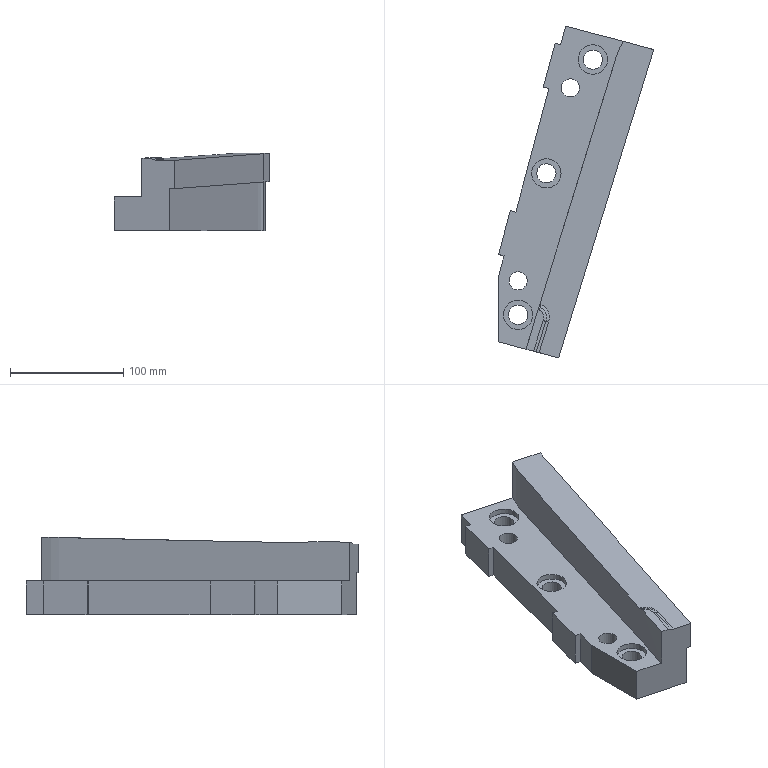Part | NX | features solid 2 | 1 solid | 40 faces | box 137.495 x 293.355 x 68.635 mm | volume 853351 mm3 | plane 17 | spline 15 | cylinder 8 | commonest cylinder face diameters 17 x3 26 x3 16 x2